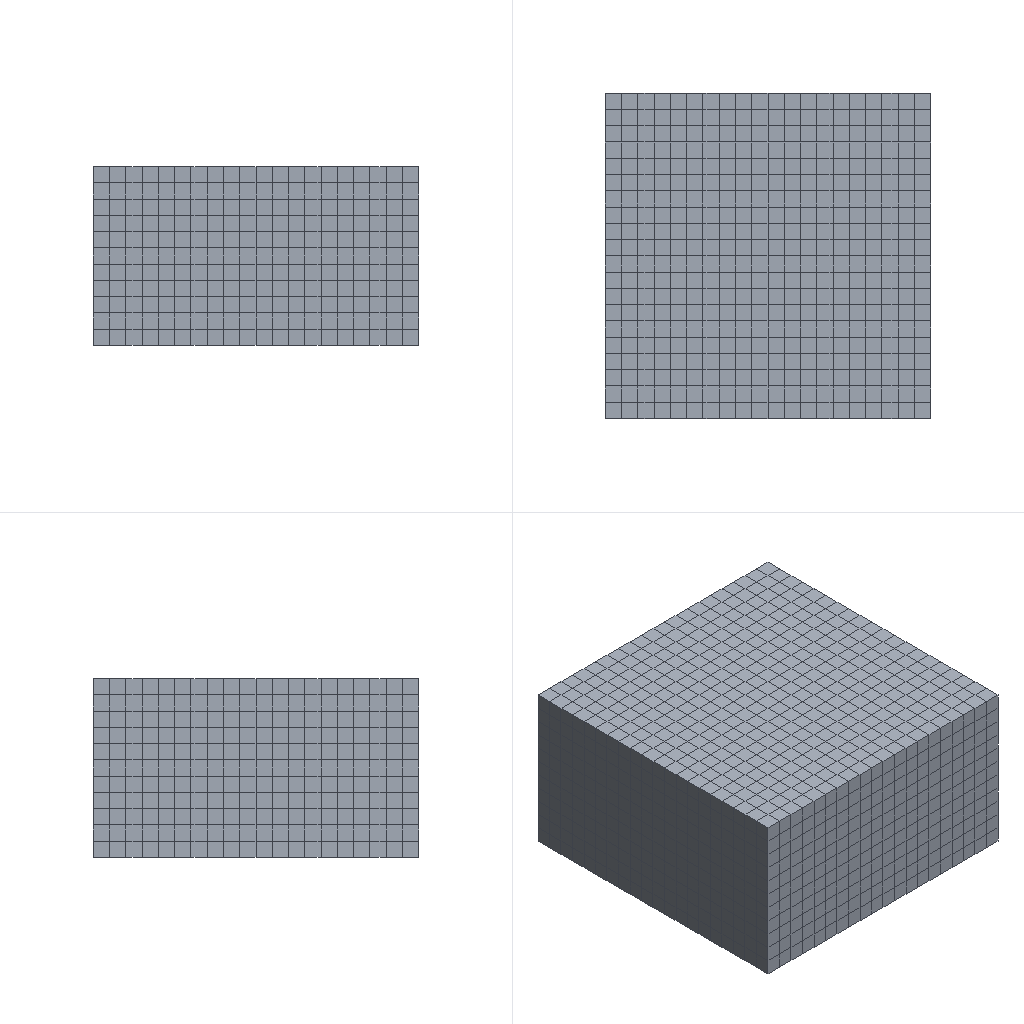Simulation study | abaqus
Set-up summary:
category,name,step,type,value,unit,region
solver,abaqus,,Abaqus/CAE 2024
units,mm-N-s-tonne (MPa),,inferred,E=69000 density=2.5e-09
analysis,Step-1,,coupled temp-displacement,nlgeom=True; time_period=3600
mesh,nodes,,,5292
mesh,elements,,,4400
element_type,C3D8T,,,4400
material,Al_1060-H16,,E,69000
material,Al_1060-H16,,nu,0
material,Al_1060-H16,,density,2.5e-09
material,Al_1060-H16,,yield,105
material,Al_1060-H16,,conductivity,30
material,Al_1060-H16,,specific_heat,4.62e+08
material,Al_1060-H16,,cte,1.31e-05
material,Al_1060-H16,,behaviors,plastic; conductivity; expansion; specific heat
material,Material-1,,E,235000
material,Material-1,,nu,0.292
material,Material-1,,density,8.72e-09
material,Material-1,,yield,300
material,Material-1,,conductivity,30
material,Material-1,,specific_heat,4.62e+08
material,Material-1,,cte,1.31e-05
material,Material-1,,behaviors,plastic; conductivity; expansion; specific heat
material,Material-2,,E,195000
material,Material-2,,nu,0.31
material,Material-2,,density,7.4e-09
material,Material-2,,yield,280
material,Material-2,,conductivity,32
material,Material-2,,specific_heat,4.8e+08
material,Material-2,,cte,1.25e-05
material,Material-2,,behaviors,plastic; conductivity; expansion; specific heat
material,Material-3,,E,190000
material,Material-3,,nu,0.32
material,Material-3,,density,7e-09
material,Material-3,,yield,310
material,Material-3,,conductivity,38
material,Material-3,,specific_heat,5e+08
material,Material-3,,cte,1.2e-05
material,Material-3,,behaviors,plastic; conductivity; expansion; specific heat
material,Material-4,,E,180000
material,Material-4,,nu,0.33
material,Material-4,,density,6.8e-09
material,Material-4,,yield,290
material,Material-4,,conductivity,42
material,Material-4,,specific_heat,520
material,Material-4,,cte,1.15e-05
material,Material-4,,behaviors,plastic; conductivity; expansion; specific heat
material,Material-5,,E,165000
material,Material-5,,nu,0.34
material,Material-5,,density,3.46e-09
material,Material-5,,yield,260
material,Material-5,,conductivity,38
material,Material-5,,specific_heat,560
material,Material-5,,cte,1.32e-05
material,Material-5,,behaviors,plastic; conductivity; expansion; specific heat
material,Material-6,,E,160000
material,Material-6,,nu,0.34
material,Material-6,,density,6.2e-09
material,Material-6,,yield,240
material,Material-6,,conductivity,48
material,Material-6,,specific_heat,540
material,Material-6,,cte,1.38e-05
material,Material-6,,behaviors,plastic; conductivity; expansion; specific heat
material,Material-7,,E,145000
material,Material-7,,nu,0.35
material,Material-7,,density,5.8e-09
material,Material-7,,yield,210
material,Material-7,,conductivity,55
material,Material-7,,specific_heat,5.6e+08
material,Material-7,,cte,1.62e-05
material,Material-7,,behaviors,plastic; conductivity; expansion; specific heat
material,Material-8,,E,130000
material,Material-8,,nu,0.36
material,Material-8,,density,5.4e-09
material,Material-8,,yield,180
material,Material-8,,conductivity,50
material,Material-8,,specific_heat,5.8e+08
material,Material-8,,cte,1.85e-05
material,Material-8,,behaviors,plastic; conductivity; expansion; specific heat
material,Material-9,,E,115000
material,Material-9,,nu,0.37
material,Material-9,,density,5.1e-09
material,Material-9,,yield,150
material,Material-9,,conductivity,70
material,Material-9,,specific_heat,6e+08
material,Material-9,,cte,2.1e-05
material,Material-9,,behaviors,plastic; conductivity; expansion; specific heat
material,Pure Nickel,,E,207000
material,Pure Nickel,,nu,0.31
material,Pure Nickel,,density,8.88e-09
material,Pure Nickel,,conductivity,60.7
material,Pure Nickel,,specific_heat,4.6e-07
material,Pure Nickel,,cte,1.31e-05
material,Pure Nickel,,behaviors,conductivity; expansion; latent heat; specific heat
section,Material-9,,solid section,,,Set-10
section,Al_1060-H16,,solid section,,,Set-11
section,Material-7,,solid section,,,Set-9
section,Material-6,,solid section,,,Set-7
section,Material-5,,solid section,,,Set-6
section,Material-4,,solid section,,,Set-5
section,Material-3,,solid section,,,Set-4
section,Material-2,,solid section,,,Set-3
section,Material-1,,solid section,,,Set-2
section,Material-7,,solid section,,,Set-8
section,Al_1060-H16,,solid section,,,Set-1
load,Predefined,initial,initial condition temperature
load,Int-1,Step-1,sfilm,0.05,,Surf-1
bc,BC-1,initial,fixed,"[dofs=rx,ry,rz,x,y,z n=6]",,Set-1
Abaqus input file, long lists of numbers shortened:
*Heading
** Job name: deck Model name: Model-1
** Generated by: Abaqus/CAE 2024
*Preprint, echo=NO, model=NO, history=NO, contact=NO
**
** PARTS
**
*Part, name=Part-10
*Node
      1,         100.,           0.,          50.
      2,           0.,           0.,          50.
** (5290 more lines like these left out)
*Element, type=C3D8T
  1,  162,  961, 1322,  125,    1,   49,   86,    4
  2,  961,  962, 1323, 1322,   49,   50,   85,   86
** (4398 more lines like these left out)
*Nset, nset=Set-1
   41,   42,   43,   44,   45,   46,   47,   48,  809,  810,  811,  812,  813,  814,  815,  816
  817,  818,  819,  820,  821,  822,  823,  824,  825,  826,  827,  828,  829,  830,  831,  832
** (54 more lines like these left out)
*Elset, elset=Set-1, generate
 4001,  4400,     1
*Nset, nset=Set-2
   37,   38,   39,   40,   41,   42,   43,   44,  733,  734,  735,  736,  737,  738,  739,  740
  741,  742,  743,  744,  745,  746,  747,  748,  749,  750,  751,  752,  753,  754,  755,  756
** (54 more lines like these left out)
*Elset, elset=Set-2, generate
 3201,  3600,     1
*Nset, nset=Set-3
   33,   34,   35,   36,   37,   38,   39,   40,  657,  658,  659,  660,  661,  662,  663,  664
  665,  666,  667,  668,  669,  670,  671,  672,  673,  674,  675,  676,  677,  678,  679,  680
** (54 more lines like these left out)
*Elset, elset=Set-3, generate
 2801,  3200,     1
*Nset, nset=Set-4
   29,   30,   31,   32,   33,   34,   35,   36,  581,  582,  583,  584,  585,  586,  587,  588
  589,  590,  591,  592,  593,  594,  595,  596,  597,  598,  599,  600,  601,  602,  603,  604
** (54 more lines like these left out)
*Elset, elset=Set-4, generate
 2401,  2800,     1
*Nset, nset=Set-5
   25,   26,   27,   28,   29,   30,   31,   32,  505,  506,  507,  508,  509,  510,  511,  512
  513,  514,  515,  516,  517,  518,  519,  520,  521,  522,  523,  524,  525,  526,  527,  528
** (54 more lines like these left out)
*Elset, elset=Set-5, generate
 2001,  2400,     1
*Nset, nset=Set-6
   17,   18,   21,   24,   25,   26,   27,   28,  353,  354,  355,  356,  357,  358,  359,  360
  361,  362,  363,  364,  365,  366,  367,  368,  369,  370,  371,  391,  392,  393,  394,  395
** (54 more lines like these left out)
*Elset, elset=Set-6, generate
 1601,  2000,     1
*Nset, nset=Set-7
   17,   18,   19,   20,   21,   22,   23,   24,  353,  354,  355,  356,  357,  358,  359,  360
  361,  362,  363,  364,  365,  366,  367,  368,  369,  370,  371,  372,  373,  374,  375,  376
** (54 more lines like these left out)
*Elset, elset=Set-7, generate
 1201,  1600,     1
*Nset, nset=Set-8
   13,   14,   15,   16,   19,   20,   22,   23,  277,  278,  279,  280,  281,  282,  283,  284
  285,  286,  287,  288,  289,  290,  291,  292,  293,  294,  295,  296,  297,  298,  299,  300
** (54 more lines like these left out)
*Elset, elset=Set-8, generate
 3601,  4000,     1
*Nset, nset=Set-9
    3,    4,    6,    7,   13,   14,   15,   16,   68,   69,   70,   71,   72,   73,   74,   75
   76,   77,   78,   79,   80,   81,   82,   83,   84,   85,   86,  106,  107,  108,  109,  110
** (54 more lines like these left out)
*Elset, elset=Set-9, generate
  801,  1200,     1
*Nset, nset=Set-10
    1,    2,    3,    4,    5,    6,    7,    8,   49,   50,   51,   52,   53,   54,   55,   56
   57,   58,   59,   60,   61,   62,   63,   64,   65,   66,   67,   68,   69,   70,   71,   72
** (54 more lines like these left out)
*Elset, elset=Set-10, generate
   1,  400,    1
*Nset, nset=Set-11
    1,    2,    5,    8,    9,   10,   11,   12,   49,   50,   51,   52,   53,   54,   55,   56
   57,   58,   59,   60,   61,   62,   63,   64,   65,   66,   67,   87,   88,   89,   90,   91
** (54 more lines like these left out)
*Elset, elset=Set-11, generate
 401,  800,    1
*Nset, nset=Set-16, generate
    1,  5292,     1
*Elset, elset=Set-16, generate
    1,  4400,     1
*Nset, nset=Set-17, generate
    1,  5292,     1
*Elset, elset=Set-17, generate
    1,  4400,     1
** Section: Section-10
*Solid Section, elset=Set-10, material=Material-9
,
** Section: Section-1
*Solid Section, elset=Set-11, material=Al_1060-H16
,
** Section: Section-8
*Solid Section, elset=Set-9, material=Material-7
,
** Section: Section-7
*Solid Section, elset=Set-7, material=Material-6
,
** Section: Section-6
*Solid Section, elset=Set-6, material=Material-5
,
** Section: Section-5
*Solid Section, elset=Set-5, material=Material-4
,
** Section: Section-4
*Solid Section, elset=Set-4, material=Material-3
,
** Section: Section-3
*Solid Section, elset=Set-3, material=Material-2
,
** Section: Section-2
*Solid Section, elset=Set-2, material=Material-1
,
** Section: Section-8
*Solid Section, elset=Set-8, material=Material-7
,
** Section: Section-1
*Solid Section, elset=Set-1, material=Al_1060-H16
,
*End Part
**
**
** ASSEMBLY
**
*Assembly, name=Assembly
**
*Instance, name=Part-10-1, part=Part-10
*End Instance
**
*Nset, nset=Set-1, instance=Part-10-1
    9,   10,   11,   12,  201,  202,  203,  204,  205,  206,  207,  208,  209,  210,  211,  212
  213,  214,  215,  216,  217,  218,  219,  220,  221,  222,  223,  224,  225,  226,  227,  228
** (26 more lines like these left out)
*Elset, elset=Set-1, instance=Part-10-1, generate
 401,  800,    1
*Nset, nset=Set-2, instance=Part-10-1, generate
    1,  5292,     1
*Elset, elset=Set-2, instance=Part-10-1, generate
    1,  4400,     1
*Elset, elset=_Surf-1_S2, internal, instance=Part-10-1
    1,    2,    3,    4,    5,    6,    7,    8,    9,   10,   11,   12,   13,   14,   15,   16
   17,   18,   19,   20,  401,  402,  403,  404,  405,  406,  407,  408,  409,  410,  411,  412
** (12 more lines like these left out)
*Elset, elset=_Surf-1_S6, internal, instance=Part-10-1, generate
    1,  4381,    20
*Elset, elset=_Surf-1_S4, internal, instance=Part-10-1, generate
   20,  4400,    20
*Elset, elset=_Surf-1_S1, internal, instance=Part-10-1
  381,  382,  383,  384,  385,  386,  387,  388,  389,  390,  391,  392,  393,  394,  395,  396
  397,  398,  399,  400,  781,  782,  783,  784,  785,  786,  787,  788,  789,  790,  791,  792
** (12 more lines like these left out)
*Elset, elset=_Surf-1_S5, internal, instance=Part-10-1
  401,  402,  403,  404,  405,  406,  407,  408,  409,  410,  411,  412,  413,  414,  415,  416
  417,  418,  419,  420,  421,  422,  423,  424,  425,  426,  427,  428,  429,  430,  431,  432
** (48 more lines like these left out)
*Surface, type=ELEMENT, name=Surf-1
_Surf-1_S2, S2
_Surf-1_S6, S6
_Surf-1_S4, S4
_Surf-1_S1, S1
_Surf-1_S5, S5
*End Assembly
**
** MATERIALS
**
*Material, name=Al_1060-H16
*Conductivity
30.,
*Density
 2.5e-09,
*Elastic
69000.,0.
*Expansion
 1.31e-05,
*Plastic
105.,0.
*Specific Heat
 4.62e+08,
*Material, name=Material-1
*Conductivity
30.,200.
34.,400.
38.,600.
*Density
 8.72e-09,
*Elastic
235000., 0.292,   25.
223600., 0.292,  100.
216000., 0.296,  200.
208400., 0.296,  300.
201000.,   0.3,  400.
193400., 0.304,  500.
186500., 0.308,  600.
180000., 0.308,  700.
*Expansion
 1.31e-05, 25.
 1.38e-05,200.
 1.45e-05,400.
 1.52e-05,600.
 1.58e-05,800.
*Plastic
  300.,    0.,   25.
  320.,  0.02,   25.
  340.,  0.05,   25.
  280.,    0.,  100.
  295., 0.025,  100.
  305.,  0.06,  100.
  250.,    0.,  200.
  260.,  0.03,  200.
  265.,  0.07,  200.
  220.,    0.,  300.
  225., 0.035,  300.
  228.,  0.08,  300.
  190.,    0.,  400.
  192.,  0.04,  400.
  194.,  0.09,  400.
  160.,    0.,  500.
  161., 0.045,  500.
  162.,   0.1,  500.
  130.,    0.,  600.
 130.5,  0.05,  600.
  131.,  0.12,  600.
  100.,    0.,  700.
 100.2,  0.06,  700.
 100.5,  0.15,  700.
   70.,    0.,  800.
  70.1,  0.08,  800.
  70.2,   0.2,  800.
*Specific Heat
 4.62e+08, 25.
    5e+08,600.
  5.3e+08,800.
*Material, name=Material-2
*Conductivity
32.,
*Density
 7.4e-09,
*Elastic
195000., 0.31
*Expansion
 1.25e-05, 25.
 1.28e-05,100.
 1.32e-05,200.
 1.36e-05,300.
 1.39e-05,400.
 1.43e-05,500.
 1.47e-05,700.
 1.55e-05,800.
*Plastic
280.,   0.
330., 0.06
*Specific Heat
 4.8e+08, 20.
   5e+08,600.
 5.3e+08,800.
*Material, name=Material-3
*Conductivity
38.,
*Density
 7e-09,
*Elastic
190000., 0.32
*Expansion
  1.2e-05, 25.
 1.27e-05,200.
 1.31e-05,300.
 1.35e-05,400.
 1.39e-05,500.
 1.47e-05,700.
 1.51e-05,800.
*Plastic
310.,   0.
360., 0.07
*Specific Heat
 5e+08,
*Material, name=Material-4
*Conductivity
42.,
*Density
 6.8e-09,
*Elastic
180000., 0.33
*Expansion
 1.15e-05, 25.
 1.18e-05,100.
 1.22e-05,200.
 1.26e-05,300.
  1.3e-05,400.
 1.34e-05,500.
 1.38e-05,600.
 1.42e-05,700.
 1.42e-05,800.
*Plastic
290.,   0.
340., 0.08
*Specific Heat
520.,
*Material, name=Material-5
*Conductivity
38.,
*Density
 3.46e-09,
*Elastic
165000., 0.34
*Expansion
 1.32e-05, 25.
 1.35e-05,100.
 1.39e-05,200.
 1.43e-05,300.
 1.48e-05,400.
 1.53e-05,500.
 1.58e-05,600.
*Plastic
260.,  0.
310., 0.1
*Specific Heat
560.,
*Material, name=Material-6
*Conductivity
48.,
*Density
 6.2e-09,
*Elastic
160000., 0.34
*Expansion
 1.38e-05, 25.
 1.42e-05,100.
 1.46e-05,200.
  1.5e-05,300.
 1.55e-05,400.
  1.6e-05,500.
 1.65e-05,600.
  1.7e-05,700.
 1.75e-05,800.
*Plastic
240.,  0.
290., 0.1
*Specific Heat
540.,
*Material, name=Material-7
*Conductivity
55., 25.
45.,700.
*Density
 5.8e-09,
*Elastic
145000., 0.35
*Expansion
 1.62e-05, 25.
 1.67e-05,100.
 1.72e-05,200.
 1.78e-05,300.
 1.84e-05,400.
  1.9e-05,500.
 1.96e-05,600.
 2.02e-05,700.
 2.08e-05,800.
*Plastic
210.,   0.
230., 0.12
*Specific Heat
 5.6e+08,
*Material, name=Material-8
*Conductivity
50., 0.
62.,25.
*Density
 5.4e-09,
*Elastic
130000., 0.36
*Expansion
 1.85e-05, 25.
 1.91e-05,100.
 1.97e-05,200.
 2.04e-05,300.
 2.11e-05,400.
 2.18e-05,500.
 2.25e-05,600.
 2.32e-05,700.
 2.39e-05,800.
*Plastic
180.,   0.
230., 0.14
*Specific Heat
 5.8e+08,
*Material, name=Material-9
*Conductivity
70., 25.
50.,800.
*Density
 5.1e-09,
*Elastic
115000., 0.37
*Expansion
  2.1e-05, 25.
 2.17e-05,100.
 2.24e-05,200.
 2.32e-05,300.
  2.4e-05,400.
 2.48e-05,500.
 2.56e-05,600.
 2.64e-05,700.
 2.72e-05,800.
*Plastic
150.,   0.,  25.
200., 0.16,  25.
160.,   0., 800.
*Specific Heat
 6e+08,
*Material, name="Pure Nickel"
*Conductivity
 60.7,
*Density
 8.88e-09,
*Elastic
207000., 0.31
*Expansion
 1.31e-05,
*Latent Heat
305600.,   0.,1455.
*Specific Heat
 4.6e-07,
**
** BOUNDARY CONDITIONS
**
** Name: BC-1 Type: Displacement/Rotation
*Boundary
Set-1, 1, 1
Set-1, 2, 2
Set-1, 3, 3
Set-1, 4, 4
Set-1, 5, 5
Set-1, 6, 6
**
** PREDEFINED FIELDS
**
** Name: Predefined Field-1   Type: Temperature
*Initial Conditions, type=TEMPERATURE
Set-2, 1200.
** ----------------------------------------------------------------
**
** STEP: Step-1
**
*Step, name=Step-1, nlgeom=YES, inc=1000
*Coupled Temperature-displacement, creep=none, deltmx=50., stabilize, factor=0.0005, allsdtol=0, continue=NO
0.001, 3600., 1e-05, 50.
**
** INTERACTIONS
**
** Interaction: Int-1
*Sfilm
Surf-1, F, 25., 0.05
**
** OUTPUT REQUESTS
**
*Restart, write, frequency=0
**
** FIELD OUTPUT: F-Output-1
**
*Output, field, frequency=10
*Node Output
NT, U
*Element Output, directions=YES
PEEQ, S
**
** HISTORY OUTPUT: H-Output-1
**
*Output, history, variable=PRESELECT
*End Step
Results summary:
result,odb.job_status,,,JOB_STATUS_COMPLETED_SUCCESSFULLY,"consistent, unstated (Abaqus has no unit system)"
result,steps[0].procedure,Step-1,,"*COUPLED TEMPERATURE-DISPLACEMENT, STEADY STATE","consistent, unstated (Abaqus has no unit system)"
result,steps[0].time_period,Step-1,,3600,"consistent, unstated (Abaqus has no unit system)"
result,steps[0].n_frames,Step-1,,11,"consistent, unstated (Abaqus has no unit system)"
result,steps[0].last_frame.id,Step-1,,99,"consistent, unstated (Abaqus has no unit system)"
result,steps[0].last_frame.value,Step-1,,3600,"consistent, unstated (Abaqus has no unit system)"
result,steps[0].last_frame.description,Step-1,,Increment     99: Step Time =    3600.,"consistent, unstated (Abaqus has no unit system)"
result,steps[0].completed,Step-1,,True,"consistent, unstated (Abaqus has no unit system)"
result,steps[0].max_U_magnitude,Step-1,,1.852,"consistent, unstated (Abaqus has no unit system)"
result,steps[0].max_S_mises,Step-1,,310.084,"consistent, unstated (Abaqus has no unit system)"